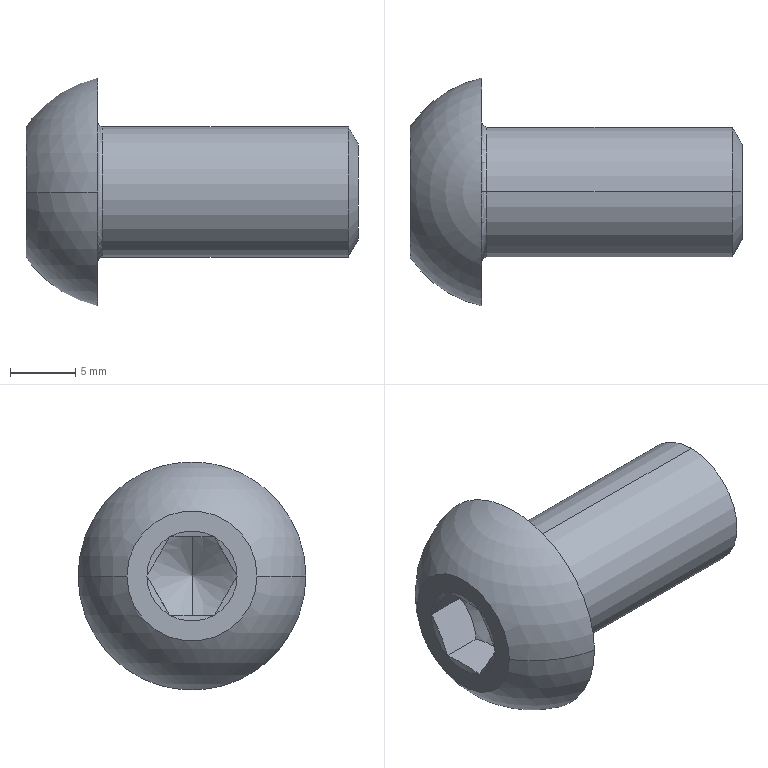Part | SolidWorks | 1 solid | 25 faces | box 25.5 x 17.5 x 17.5 mm | volume 2396 mm3 | cone 10 | plane 9 | torus 2 | sphere 2 | cylinder 2 | commonest cylinder face diameters 10 x2
STEP:
#1=CARTESIAN_POINT('',(0.,0.,3.701));
#2=VERTEX_POINT('',#1);
#3=CARTESIAN_POINT('',(0.,0.,-3.701));
#4=VERTEX_POINT('',#3);
#5=CARTESIAN_POINT('',(0.,0.,0.));
#6=DIRECTION('',(-1.,0.,0.));
#7=DIRECTION('',(0.,0.,1.));
#8=AXIS2_PLACEMENT_3D('',#5,#6,#7);
#9=CIRCLE('',#8,3.701);
#10=EDGE_CURVE('',#2,#4,#9,.T.);
#11=ORIENTED_EDGE('',*,*,#10,.T.);
#12=CARTESIAN_POINT('',(-0.75,0.,-5.));
#13=VERTEX_POINT('',#12);
#14=CARTESIAN_POINT('',(-0.75,0.,-5.));
#15=DIRECTION('',(-0.5,0.,-0.866));
#16=VECTOR('',#15,1000.);
#17=LINE('',#14,#16);
#18=EDGE_CURVE('',#4,#13,#17,.T.);
#19=ORIENTED_EDGE('',*,*,#18,.T.);
#20=CARTESIAN_POINT('',(-0.75,0.,5.));
#21=VERTEX_POINT('',#20);
#22=CARTESIAN_POINT('',(-0.75,0.,0.));
#23=DIRECTION('',(-1.,0.,0.));
#24=DIRECTION('',(0.,0.,1.));
#25=AXIS2_PLACEMENT_3D('',#22,#23,#24);
#26=CIRCLE('',#25,5.);
#27=EDGE_CURVE('',#21,#13,#26,.T.);
#28=ORIENTED_EDGE('',*,*,#27,.F.);
#29=CARTESIAN_POINT('',(-0.75,0.,5.));
#30=DIRECTION('',(-0.5,0.,0.866));
#31=VECTOR('',#30,1000.);
#32=LINE('',#29,#31);
#33=EDGE_CURVE('',#2,#21,#32,.T.);
#34=ORIENTED_EDGE('',*,*,#33,.F.);
#35=EDGE_LOOP('',(#11,#19,#28,#34));
#36=FACE_OUTER_BOUND('',#35,.T.);
#37=CARTESIAN_POINT('',(-0.75,0.,0.));
#38=DIRECTION('',(-1.,0.,0.));
#39=DIRECTION('',(0.,0.,1.));
#40=AXIS2_PLACEMENT_3D('',#37,#38,#39);
#41=CONICAL_SURFACE('',#40,5.,1.047);
#42=ADVANCED_FACE('',(#36),#41,.T.);
#43=CARTESIAN_POINT('',(-20.,0.,0.));
#44=VERTEX_POINT('',#43);
#45=CARTESIAN_POINT('',(-22.061,0.,3.));
#46=VERTEX_POINT('',#45);
#47=CARTESIAN_POINT('',(-22.38,0.,3.464));
#48=DIRECTION('',(-0.5663,0.,0.8242));
#49=VECTOR('',#48,1000.);
#50=LINE('',#47,#49);
#51=EDGE_CURVE('',#44,#46,#50,.T.);
#52=ORIENTED_EDGE('',*,*,#51,.F.);
#53=CARTESIAN_POINT('',(-22.061,0.,-3.));
#54=VERTEX_POINT('',#53);
#55=CARTESIAN_POINT('',(-22.38,0.,-3.464));
#56=DIRECTION('',(-0.5663,0.,-0.8242));
#57=VECTOR('',#56,1000.);
#58=LINE('',#55,#57);
#59=EDGE_CURVE('',#44,#54,#58,.T.);
#60=ORIENTED_EDGE('',*,*,#59,.T.);
#61=CARTESIAN_POINT('',(-22.38,-1.732,-3.));
#62=VERTEX_POINT('',#61);
#63=CARTESIAN_POINT('',(-22.061,0.,-3.));
#64=CARTESIAN_POINT('',(-22.061,-0.2941,-3.));
#65=CARTESIAN_POINT('',(-22.091,-0.5858,-3.));
#66=CARTESIAN_POINT('',(-22.203,-1.166,-3.));
#67=CARTESIAN_POINT('',(-22.284,-1.453,-3.));
#68=CARTESIAN_POINT('',(-22.38,-1.732,-3.));
#69=B_SPLINE_CURVE_WITH_KNOTS('',3,(#63,#64,#65,#66,#67,#68),.UNSPECIFIED.,.F.,.F.,(4,2,4),(0.01073,0.01162,0.0125),.UNSPECIFIED.);
#70=EDGE_CURVE('',#54,#62,#69,.T.);
#71=ORIENTED_EDGE('',*,*,#70,.T.);
#72=CARTESIAN_POINT('',(-22.38,-3.464,0.));
#73=VERTEX_POINT('',#72);
#74=CARTESIAN_POINT('',(-22.38,-1.732,-3.));
#75=CARTESIAN_POINT('',(-22.187,-2.012,-2.514));
#76=CARTESIAN_POINT('',(-22.062,-2.299,-2.019));
#77=CARTESIAN_POINT('',(-22.061,-2.669,-1.377));
#78=CARTESIAN_POINT('',(-22.068,-2.744,-1.247));
#79=CARTESIAN_POINT('',(-22.098,-2.891,-0.9922));
#80=CARTESIAN_POINT('',(-22.12,-2.964,-0.8658));
#81=CARTESIAN_POINT('',(-22.203,-3.181,-0.4899));
#82=CARTESIAN_POINT('',(-22.283,-3.324,-0.2435));
#83=CARTESIAN_POINT('',(-22.38,-3.464,0.));
#84=B_SPLINE_CURVE_WITH_KNOTS('',3,(#74,#75,#76,#77,#78,#79,#80,#81,#82,#83),.UNSPECIFIED.,.F.,.F.,(4,2,2,2,4),(0.000000241,0.001755,0.002194,0.002632,0.00351),.UNSPECIFIED.);
#85=EDGE_CURVE('',#62,#73,#84,.T.);
#86=ORIENTED_EDGE('',*,*,#85,.T.);
#87=CARTESIAN_POINT('',(-22.38,-1.732,3.));
#88=VERTEX_POINT('',#87);
#89=CARTESIAN_POINT('',(-22.38,-3.464,0.));
#90=CARTESIAN_POINT('',(-22.187,-3.184,0.4857));
#91=CARTESIAN_POINT('',(-22.062,-2.898,0.9812));
#92=CARTESIAN_POINT('',(-22.061,-2.527,1.623));
#93=CARTESIAN_POINT('',(-22.068,-2.452,1.753));
#94=CARTESIAN_POINT('',(-22.098,-2.305,2.008));
#95=CARTESIAN_POINT('',(-22.12,-2.232,2.134));
#96=CARTESIAN_POINT('',(-22.203,-2.015,2.51));
#97=CARTESIAN_POINT('',(-22.283,-1.873,2.756));
#98=CARTESIAN_POINT('',(-22.38,-1.732,3.));
#99=B_SPLINE_CURVE_WITH_KNOTS('',3,(#89,#90,#91,#92,#93,#94,#95,#96,#97,#98),.UNSPECIFIED.,.F.,.F.,(4,2,2,2,4),(0.000000241,0.001755,0.002194,0.002632,0.00351),.UNSPECIFIED.);
#100=EDGE_CURVE('',#73,#88,#99,.T.);
#101=ORIENTED_EDGE('',*,*,#100,.T.);
#102=CARTESIAN_POINT('',(-22.38,-1.732,3.));
#103=CARTESIAN_POINT('',(-22.284,-1.453,3.));
#104=CARTESIAN_POINT('',(-22.203,-1.166,3.));
#105=CARTESIAN_POINT('',(-22.091,-0.5858,3.));
#106=CARTESIAN_POINT('',(-22.061,-0.2941,3.));
#107=CARTESIAN_POINT('',(-22.061,0.,3.));
#108=B_SPLINE_CURVE_WITH_KNOTS('',3,(#102,#103,#104,#105,#106,#107),.UNSPECIFIED.,.F.,.F.,(4,2,4),(0.002487,0.003368,0.00425),.UNSPECIFIED.);
#109=EDGE_CURVE('',#88,#46,#108,.T.);
#110=ORIENTED_EDGE('',*,*,#109,.T.);
#111=EDGE_LOOP('',(#52,#60,#71,#86,#101,#110));
#112=FACE_OUTER_BOUND('',#111,.T.);
#113=CARTESIAN_POINT('',(-22.38,0.,0.));
#114=DIRECTION('',(-1.,0.,0.));
#115=DIRECTION('',(0.,0.,1.));
#116=AXIS2_PLACEMENT_3D('',#113,#114,#115);
#117=CONICAL_SURFACE('',#116,3.464,0.9688);
#118=ADVANCED_FACE('',(#112),#117,.F.);
#119=CARTESIAN_POINT('',(-20.,0.,-5.4));
#120=VERTEX_POINT('',#119);
#121=CARTESIAN_POINT('',(-20.,0.,5.4));
#122=VERTEX_POINT('',#121);
#123=CARTESIAN_POINT('',(-20.,0.,0.));
#124=DIRECTION('',(-1.,0.,0.));
#125=DIRECTION('',(0.,0.,1.));
#126=AXIS2_PLACEMENT_3D('',#123,#124,#125);
#127=CIRCLE('',#126,5.4);
#128=EDGE_CURVE('',#120,#122,#127,.T.);
#129=ORIENTED_EDGE('',*,*,#128,.F.);
#130=CARTESIAN_POINT('',(-19.6,0.,-5.));
#131=VERTEX_POINT('',#130);
#132=CARTESIAN_POINT('',(-19.6,0.,-5.4));
#133=DIRECTION('',(0.,1.,0.));
#134=DIRECTION('',(0.,0.,1.));
#135=AXIS2_PLACEMENT_3D('',#132,#133,#134);
#136=CIRCLE('',#135,0.4);
#137=EDGE_CURVE('',#120,#131,#136,.T.);
#138=ORIENTED_EDGE('',*,*,#137,.T.);
#139=CARTESIAN_POINT('',(-19.6,0.,5.));
#140=VERTEX_POINT('',#139);
#141=CARTESIAN_POINT('',(-19.6,0.,0.));
#142=DIRECTION('',(-1.,0.,0.));
#143=DIRECTION('',(0.,0.,1.));
#144=AXIS2_PLACEMENT_3D('',#141,#142,#143);
#145=CIRCLE('',#144,5.);
#146=EDGE_CURVE('',#131,#140,#145,.T.);
#147=ORIENTED_EDGE('',*,*,#146,.T.);
#148=CARTESIAN_POINT('',(-19.6,0.,5.4));
#149=DIRECTION('',(0.,-1.,0.));
#150=DIRECTION('',(0.,0.,-1.));
#151=AXIS2_PLACEMENT_3D('',#148,#149,#150);
#152=CIRCLE('',#151,0.4);
#153=EDGE_CURVE('',#122,#140,#152,.T.);
#154=ORIENTED_EDGE('',*,*,#153,.F.);
#155=EDGE_LOOP('',(#129,#138,#147,#154));
#156=FACE_OUTER_BOUND('',#155,.T.);
#157=CARTESIAN_POINT('',(-19.6,0.,0.));
#158=DIRECTION('',(-1.,0.,0.));
#159=DIRECTION('',(0.,0.,1.));
#160=AXIS2_PLACEMENT_3D('',#157,#158,#159);
#161=TOROIDAL_SURFACE('',#160,5.4,0.4);
#162=ADVANCED_FACE('',(#156),#161,.F.);
#163=CARTESIAN_POINT('',(-20.,8.75,0.));
#164=VERTEX_POINT('',#163);
#165=CARTESIAN_POINT('',(-20.,-8.75,0.));
#166=VERTEX_POINT('',#165);
#167=CARTESIAN_POINT('',(-20.,0.,0.));
#168=DIRECTION('',(-1.,0.,0.));
#169=DIRECTION('',(0.,0.,1.));
#170=AXIS2_PLACEMENT_3D('',#167,#168,#169);
#171=CIRCLE('',#170,8.75);
#172=EDGE_CURVE('',#164,#166,#171,.T.);
#173=ORIENTED_EDGE('',*,*,#172,.T.);
#174=CARTESIAN_POINT('',(-25.5,-5.,0.));
#175=VERTEX_POINT('',#174);
#176=CARTESIAN_POINT('',(-18.062,0.,0.));
#177=DIRECTION('',(0.,0.,-1.));
#178=DIRECTION('',(0.,1.,0.));
#179=AXIS2_PLACEMENT_3D('',#176,#177,#178);
#180=CIRCLE('',#179,8.962);
#181=EDGE_CURVE('',#166,#175,#180,.T.);
#182=ORIENTED_EDGE('',*,*,#181,.T.);
#183=CARTESIAN_POINT('',(-25.5,5.,0.));
#184=VERTEX_POINT('',#183);
#185=CARTESIAN_POINT('',(-25.5,0.,0.));
#186=DIRECTION('',(-1.,0.,0.));
#187=DIRECTION('',(0.,0.,1.));
#188=AXIS2_PLACEMENT_3D('',#185,#186,#187);
#189=CIRCLE('',#188,5.);
#190=EDGE_CURVE('',#184,#175,#189,.T.);
#191=ORIENTED_EDGE('',*,*,#190,.F.);
#192=CARTESIAN_POINT('',(-18.062,0.,0.));
#193=DIRECTION('',(0.,0.,1.));
#194=DIRECTION('',(1.,0.,0.));
#195=AXIS2_PLACEMENT_3D('',#192,#193,#194);
#196=CIRCLE('',#195,8.962);
#197=EDGE_CURVE('',#164,#184,#196,.T.);
#198=ORIENTED_EDGE('',*,*,#197,.F.);
#199=EDGE_LOOP('',(#173,#182,#191,#198));
#200=FACE_OUTER_BOUND('',#199,.T.);
#201=CARTESIAN_POINT('',(-18.062,0.,0.));
#202=DIRECTION('',(0.,0.,-1.));
#203=DIRECTION('',(0.,1.,0.));
#204=AXIS2_PLACEMENT_3D('',#201,#202,#203);
#205=SPHERICAL_SURFACE('',#204,8.962);
#206=ADVANCED_FACE('',(#200),#205,.T.);
#207=ORIENTED_EDGE('',*,*,#27,.T.);
#208=CARTESIAN_POINT('',(-25.5,0.,-5.));
#209=DIRECTION('',(-1.,0.,0.));
#210=VECTOR('',#209,1000.);
#211=LINE('',#208,#210);
#212=EDGE_CURVE('',#13,#131,#211,.T.);
#213=ORIENTED_EDGE('',*,*,#212,.T.);
#214=CARTESIAN_POINT('',(-19.6,0.,0.));
#215=DIRECTION('',(-1.,0.,0.));
#216=DIRECTION('',(0.,0.,1.));
#217=AXIS2_PLACEMENT_3D('',#214,#215,#216);
#218=CIRCLE('',#217,5.);
#219=EDGE_CURVE('',#140,#131,#218,.T.);
#220=ORIENTED_EDGE('',*,*,#219,.F.);
#221=CARTESIAN_POINT('',(-25.5,0.,5.));
#222=DIRECTION('',(-1.,0.,0.));
#223=VECTOR('',#222,1000.);
#224=LINE('',#221,#223);
#225=EDGE_CURVE('',#21,#140,#224,.T.);
#226=ORIENTED_EDGE('',*,*,#225,.F.);
#227=EDGE_LOOP('',(#207,#213,#220,#226));
#228=FACE_OUTER_BOUND('',#227,.T.);
#229=CARTESIAN_POINT('',(-25.5,0.,0.));
#230=DIRECTION('',(-1.,0.,0.));
#231=DIRECTION('',(0.,0.,1.));
#232=AXIS2_PLACEMENT_3D('',#229,#230,#231);
#233=CYLINDRICAL_SURFACE('',#232,5.);
#234=ADVANCED_FACE('',(#228),#233,.T.);
#235=ORIENTED_EDGE('',*,*,#212,.F.);
#236=CARTESIAN_POINT('',(-0.75,0.,0.));
#237=DIRECTION('',(-1.,0.,0.));
#238=DIRECTION('',(0.,0.,1.));
#239=AXIS2_PLACEMENT_3D('',#236,#237,#238);
#240=CIRCLE('',#239,5.);
#241=EDGE_CURVE('',#13,#21,#240,.T.);
#242=ORIENTED_EDGE('',*,*,#241,.T.);
#243=ORIENTED_EDGE('',*,*,#225,.T.);
#244=ORIENTED_EDGE('',*,*,#146,.F.);
#245=EDGE_LOOP('',(#235,#242,#243,#244));
#246=FACE_OUTER_BOUND('',#245,.T.);
#247=CARTESIAN_POINT('',(-25.5,0.,0.));
#248=DIRECTION('',(-1.,0.,0.));
#249=DIRECTION('',(0.,0.,1.));
#250=AXIS2_PLACEMENT_3D('',#247,#248,#249);
#251=CYLINDRICAL_SURFACE('',#250,5.);
#252=ADVANCED_FACE('',(#246),#251,.T.);
#253=ORIENTED_EDGE('',*,*,#190,.T.);
#254=CARTESIAN_POINT('',(-25.5,0.,0.));
#255=DIRECTION('',(-1.,0.,0.));
#256=DIRECTION('',(0.,0.,1.));
#257=AXIS2_PLACEMENT_3D('',#254,#255,#256);
#258=CIRCLE('',#257,5.);
#259=EDGE_CURVE('',#175,#184,#258,.T.);
#260=ORIENTED_EDGE('',*,*,#259,.T.);
#261=EDGE_LOOP('',(#253,#260));
#262=FACE_OUTER_BOUND('',#261,.T.);
#263=CARTESIAN_POINT('',(-25.5,-1.732,-3.));
#264=VERTEX_POINT('',#263);
#265=CARTESIAN_POINT('',(-25.5,-3.464,0.));
#266=VERTEX_POINT('',#265);
#267=CARTESIAN_POINT('',(-25.5,0.,0.));
#268=DIRECTION('',(-1.,0.,0.));
#269=DIRECTION('',(0.,0.,-1.));
#270=AXIS2_PLACEMENT_3D('',#267,#268,#269);
#271=CIRCLE('',#270,3.464);
#272=EDGE_CURVE('',#264,#266,#271,.T.);
#273=ORIENTED_EDGE('',*,*,#272,.F.);
#274=CARTESIAN_POINT('',(-25.5,1.732,-3.));
#275=VERTEX_POINT('',#274);
#276=CARTESIAN_POINT('',(-25.5,0.,0.));
#277=DIRECTION('',(-1.,0.,0.));
#278=DIRECTION('',(0.,0.,-1.));
#279=AXIS2_PLACEMENT_3D('',#276,#277,#278);
#280=CIRCLE('',#279,3.464);
#281=EDGE_CURVE('',#275,#264,#280,.T.);
#282=ORIENTED_EDGE('',*,*,#281,.F.);
#283=CARTESIAN_POINT('',(-25.5,3.464,0.));
#284=VERTEX_POINT('',#283);
#285=CARTESIAN_POINT('',(-25.5,0.,0.));
#286=DIRECTION('',(-1.,0.,0.));
#287=DIRECTION('',(0.,0.,-1.));
#288=AXIS2_PLACEMENT_3D('',#285,#286,#287);
#289=CIRCLE('',#288,3.464);
#290=EDGE_CURVE('',#284,#275,#289,.T.);
#291=ORIENTED_EDGE('',*,*,#290,.F.);
#292=CARTESIAN_POINT('',(-25.5,1.732,3.));
#293=VERTEX_POINT('',#292);
#294=CARTESIAN_POINT('',(-25.5,0.,0.));
#295=DIRECTION('',(-1.,0.,0.));
#296=DIRECTION('',(0.,0.,-1.));
#297=AXIS2_PLACEMENT_3D('',#294,#295,#296);
#298=CIRCLE('',#297,3.464);
#299=EDGE_CURVE('',#293,#284,#298,.T.);
#300=ORIENTED_EDGE('',*,*,#299,.F.);
#301=CARTESIAN_POINT('',(-25.5,-1.732,3.));
#302=VERTEX_POINT('',#301);
#303=CARTESIAN_POINT('',(-25.5,0.,0.));
#304=DIRECTION('',(-1.,0.,0.));
#305=DIRECTION('',(0.,0.,-1.));
#306=AXIS2_PLACEMENT_3D('',#303,#304,#305);
#307=CIRCLE('',#306,3.464);
#308=EDGE_CURVE('',#302,#293,#307,.T.);
#309=ORIENTED_EDGE('',*,*,#308,.F.);
#310=CARTESIAN_POINT('',(-25.5,0.,0.));
#311=DIRECTION('',(-1.,0.,0.));
#312=DIRECTION('',(0.,-1.,0.));
#313=AXIS2_PLACEMENT_3D('',#310,#311,#312);
#314=CIRCLE('',#313,3.464);
#315=EDGE_CURVE('',#266,#302,#314,.T.);
#316=ORIENTED_EDGE('',*,*,#315,.F.);
#317=EDGE_LOOP('',(#273,#282,#291,#300,#309,#316));
#318=FACE_BOUND('',#317,.T.);
#319=CARTESIAN_POINT('',(-25.5,0.,0.));
#320=DIRECTION('',(1.,0.,0.));
#321=DIRECTION('',(0.,0.,-1.));
#322=AXIS2_PLACEMENT_3D('',#319,#320,#321);
#323=PLANE('',#322);
#324=ADVANCED_FACE('',(#262,#318),#323,.F.);
#325=ORIENTED_EDGE('',*,*,#181,.F.);
#326=CARTESIAN_POINT('',(-20.,0.,0.));
#327=DIRECTION('',(-1.,0.,0.));
#328=DIRECTION('',(0.,0.,1.));
#329=AXIS2_PLACEMENT_3D('',#326,#327,#328);
#330=CIRCLE('',#329,8.75);
#331=EDGE_CURVE('',#166,#164,#330,.T.);
#332=ORIENTED_EDGE('',*,*,#331,.T.);
#333=ORIENTED_EDGE('',*,*,#197,.T.);
#334=ORIENTED_EDGE('',*,*,#259,.F.);
#335=EDGE_LOOP('',(#325,#332,#333,#334));
#336=FACE_OUTER_BOUND('',#335,.T.);
#337=CARTESIAN_POINT('',(-18.062,0.,0.));
#338=DIRECTION('',(0.,0.,-1.));
#339=DIRECTION('',(0.,1.,0.));
#340=AXIS2_PLACEMENT_3D('',#337,#338,#339);
#341=SPHERICAL_SURFACE('',#340,8.962);
#342=ADVANCED_FACE('',(#336),#341,.T.);
#343=ORIENTED_EDGE('',*,*,#172,.F.);
#344=ORIENTED_EDGE('',*,*,#331,.F.);
#345=EDGE_LOOP('',(#343,#344));
#346=FACE_OUTER_BOUND('',#345,.T.);
#347=CARTESIAN_POINT('',(-20.,0.,0.));
#348=DIRECTION('',(-1.,0.,0.));
#349=DIRECTION('',(0.,0.,1.));
#350=AXIS2_PLACEMENT_3D('',#347,#348,#349);
#351=CIRCLE('',#350,5.4);
#352=EDGE_CURVE('',#122,#120,#351,.T.);
#353=ORIENTED_EDGE('',*,*,#352,.T.);
#354=ORIENTED_EDGE('',*,*,#128,.T.);
#355=EDGE_LOOP('',(#353,#354));
#356=FACE_BOUND('',#355,.T.);
#357=CARTESIAN_POINT('',(-20.,5.4,0.));
#358=DIRECTION('',(-1.,0.,0.));
#359=DIRECTION('',(0.,0.,1.));
#360=AXIS2_PLACEMENT_3D('',#357,#358,#359);
#361=PLANE('',#360);
#362=ADVANCED_FACE('',(#346,#356),#361,.F.);
#363=ORIENTED_EDGE('',*,*,#137,.F.);
#364=ORIENTED_EDGE('',*,*,#352,.F.);
#365=ORIENTED_EDGE('',*,*,#153,.T.);
#366=ORIENTED_EDGE('',*,*,#219,.T.);
#367=EDGE_LOOP('',(#363,#364,#365,#366));
#368=FACE_OUTER_BOUND('',#367,.T.);
#369=CARTESIAN_POINT('',(-19.6,0.,0.));
#370=DIRECTION('',(-1.,0.,0.));
#371=DIRECTION('',(0.,0.,1.));
#372=AXIS2_PLACEMENT_3D('',#369,#370,#371);
#373=TOROIDAL_SURFACE('',#372,5.4,0.4);
#374=ADVANCED_FACE('',(#368),#373,.F.);
#375=CARTESIAN_POINT('',(-25.5,-1.732,-3.));
#376=CARTESIAN_POINT('',(-25.428,-1.155,-3.));
#377=CARTESIAN_POINT('',(-25.385,-0.5749,-3.));
#378=CARTESIAN_POINT('',(-25.385,0.5803,-3.));
#379=CARTESIAN_POINT('',(-25.429,1.157,-3.));
#380=CARTESIAN_POINT('',(-25.5,1.732,-3.));
#381=B_SPLINE_CURVE_WITH_KNOTS('',3,(#375,#376,#377,#378,#379,#380),.UNSPECIFIED.,.F.,.F.,(4,2,4),(0.002838,0.00458,0.006321),.UNSPECIFIED.);
#382=EDGE_CURVE('',#264,#275,#381,.T.);
#383=ORIENTED_EDGE('',*,*,#382,.T.);
#384=ORIENTED_EDGE('',*,*,#281,.T.);
#385=EDGE_LOOP('',(#383,#384));
#386=FACE_OUTER_BOUND('',#385,.T.);
#387=CARTESIAN_POINT('',(-1024.64,0.,0.));
#388=DIRECTION('',(-1.,0.,0.));
#389=DIRECTION('',(0.,-1.,0.));
#390=AXIS2_PLACEMENT_3D('',#387,#388,#389);
#391=CONICAL_SURFACE('',#390,4028.025,1.327);
#392=ADVANCED_FACE('',(#386),#391,.F.);
#393=CARTESIAN_POINT('',(-25.5,1.732,-3.));
#394=CARTESIAN_POINT('',(-25.428,2.021,-2.5));
#395=CARTESIAN_POINT('',(-25.341,2.598,-1.5));
#396=CARTESIAN_POINT('',(-25.428,3.175,-0.5));
#397=CARTESIAN_POINT('',(-25.5,3.464,0.));
#398=B_SPLINE_CURVE_WITH_KNOTS('',3,(#393,#394,#395,#396,#397),.UNSPECIFIED.,.F.,.F.,(4,1,4),(0.000000231,0.001732,0.003464),.UNSPECIFIED.);
#399=EDGE_CURVE('',#275,#284,#398,.T.);
#400=ORIENTED_EDGE('',*,*,#399,.T.);
#401=ORIENTED_EDGE('',*,*,#290,.T.);
#402=EDGE_LOOP('',(#400,#401));
#403=FACE_OUTER_BOUND('',#402,.T.);
#404=CARTESIAN_POINT('',(-1024.64,0.,0.));
#405=DIRECTION('',(-1.,0.,0.));
#406=DIRECTION('',(0.,-1.,0.));
#407=AXIS2_PLACEMENT_3D('',#404,#405,#406);
#408=CONICAL_SURFACE('',#407,4028.025,1.327);
#409=ADVANCED_FACE('',(#403),#408,.F.);
#410=CARTESIAN_POINT('',(-25.5,3.464,0.));
#411=CARTESIAN_POINT('',(-25.428,3.175,0.5));
#412=CARTESIAN_POINT('',(-25.341,2.598,1.5));
#413=CARTESIAN_POINT('',(-25.428,2.021,2.5));
#414=CARTESIAN_POINT('',(-25.5,1.732,3.));
#415=B_SPLINE_CURVE_WITH_KNOTS('',3,(#410,#411,#412,#413,#414),.UNSPECIFIED.,.F.,.F.,(4,1,4),(0.000000231,0.001732,0.003464),.UNSPECIFIED.);
#416=EDGE_CURVE('',#284,#293,#415,.T.);
#417=ORIENTED_EDGE('',*,*,#416,.T.);
#418=ORIENTED_EDGE('',*,*,#299,.T.);
#419=EDGE_LOOP('',(#417,#418));
#420=FACE_OUTER_BOUND('',#419,.T.);
#421=CARTESIAN_POINT('',(-1024.64,0.,0.));
#422=DIRECTION('',(-1.,0.,0.));
#423=DIRECTION('',(0.,-1.,0.));
#424=AXIS2_PLACEMENT_3D('',#421,#422,#423);
#425=CONICAL_SURFACE('',#424,4028.025,1.327);
#426=ADVANCED_FACE('',(#420),#425,.F.);
#427=CARTESIAN_POINT('',(-25.5,1.732,3.));
#428=CARTESIAN_POINT('',(-25.429,1.157,3.));
#429=CARTESIAN_POINT('',(-25.385,0.5803,3.));
#430=CARTESIAN_POINT('',(-25.385,-0.5749,3.));
#431=CARTESIAN_POINT('',(-25.428,-1.155,3.));
#432=CARTESIAN_POINT('',(-25.5,-1.732,3.));
#433=B_SPLINE_CURVE_WITH_KNOTS('',3,(#427,#428,#429,#430,#431,#432),.UNSPECIFIED.,.F.,.F.,(4,2,4),(0.007099,0.008838,0.01058),.UNSPECIFIED.);
#434=EDGE_CURVE('',#293,#302,#433,.T.);
#435=ORIENTED_EDGE('',*,*,#434,.T.);
#436=ORIENTED_EDGE('',*,*,#308,.T.);
#437=EDGE_LOOP('',(#435,#436));
#438=FACE_OUTER_BOUND('',#437,.T.);
#439=CARTESIAN_POINT('',(-1024.64,0.,0.));
#440=DIRECTION('',(-1.,0.,0.));
#441=DIRECTION('',(0.,-1.,0.));
#442=AXIS2_PLACEMENT_3D('',#439,#440,#441);
#443=CONICAL_SURFACE('',#442,4028.025,1.327);
#444=ADVANCED_FACE('',(#438),#443,.F.);
#445=CARTESIAN_POINT('',(-25.5,-1.732,3.));
#446=CARTESIAN_POINT('',(-25.428,-2.021,2.5));
#447=CARTESIAN_POINT('',(-25.341,-2.598,1.5));
#448=CARTESIAN_POINT('',(-25.428,-3.175,0.5));
#449=CARTESIAN_POINT('',(-25.5,-3.464,0.));
#450=B_SPLINE_CURVE_WITH_KNOTS('',3,(#445,#446,#447,#448,#449),.UNSPECIFIED.,.F.,.F.,(4,1,4),(0.000000231,0.001732,0.003464),.UNSPECIFIED.);
#451=EDGE_CURVE('',#302,#266,#450,.T.);
#452=ORIENTED_EDGE('',*,*,#451,.T.);
#453=ORIENTED_EDGE('',*,*,#315,.T.);
#454=EDGE_LOOP('',(#452,#453));
#455=FACE_OUTER_BOUND('',#454,.T.);
#456=CARTESIAN_POINT('',(-1024.64,0.,0.));
#457=DIRECTION('',(-1.,0.,0.));
#458=DIRECTION('',(0.,-1.,0.));
#459=AXIS2_PLACEMENT_3D('',#456,#457,#458);
#460=CONICAL_SURFACE('',#459,4028.025,1.327);
#461=ADVANCED_FACE('',(#455),#460,.F.);
#462=CARTESIAN_POINT('',(-25.5,-3.464,0.));
#463=CARTESIAN_POINT('',(-25.428,-3.175,-0.5));
#464=CARTESIAN_POINT('',(-25.341,-2.598,-1.5));
#465=CARTESIAN_POINT('',(-25.428,-2.021,-2.5));
#466=CARTESIAN_POINT('',(-25.5,-1.732,-3.));
#467=B_SPLINE_CURVE_WITH_KNOTS('',3,(#462,#463,#464,#465,#466),.UNSPECIFIED.,.F.,.F.,(4,1,4),(0.000000231,0.001732,0.003464),.UNSPECIFIED.);
#468=EDGE_CURVE('',#266,#264,#467,.T.);
#469=ORIENTED_EDGE('',*,*,#468,.T.);
#470=ORIENTED_EDGE('',*,*,#272,.T.);
#471=EDGE_LOOP('',(#469,#470));
#472=FACE_OUTER_BOUND('',#471,.T.);
#473=CARTESIAN_POINT('',(-1024.64,0.,0.));
#474=DIRECTION('',(-1.,0.,0.));
#475=DIRECTION('',(0.,-1.,0.));
#476=AXIS2_PLACEMENT_3D('',#473,#474,#475);
#477=CONICAL_SURFACE('',#476,4028.025,1.327);
#478=ADVANCED_FACE('',(#472),#477,.F.);
#479=ORIENTED_EDGE('',*,*,#59,.F.);
#480=ORIENTED_EDGE('',*,*,#51,.T.);
#481=CARTESIAN_POINT('',(-22.38,1.732,3.));
#482=VERTEX_POINT('',#481);
#483=CARTESIAN_POINT('',(-22.061,0.,3.));
#484=CARTESIAN_POINT('',(-22.061,0.2938,3.));
#485=CARTESIAN_POINT('',(-22.092,0.5926,3.));
#486=CARTESIAN_POINT('',(-22.205,1.172,3.));
#487=CARTESIAN_POINT('',(-22.285,1.454,3.));
#488=CARTESIAN_POINT('',(-22.38,1.732,3.));
#489=B_SPLINE_CURVE_WITH_KNOTS('',3,(#483,#484,#485,#486,#487,#488),.UNSPECIFIED.,.F.,.F.,(4,2,4),(0.00425,0.00513,0.00601),.UNSPECIFIED.);
#490=EDGE_CURVE('',#46,#482,#489,.T.);
#491=ORIENTED_EDGE('',*,*,#490,.T.);
#492=CARTESIAN_POINT('',(-22.38,3.464,0.));
#493=VERTEX_POINT('',#492);
#494=CARTESIAN_POINT('',(-22.38,1.732,3.));
#495=CARTESIAN_POINT('',(-22.187,2.012,2.514));
#496=CARTESIAN_POINT('',(-22.062,2.299,2.019));
#497=CARTESIAN_POINT('',(-22.061,2.669,1.377));
#498=CARTESIAN_POINT('',(-22.068,2.744,1.247));
#499=CARTESIAN_POINT('',(-22.098,2.891,0.9922));
#500=CARTESIAN_POINT('',(-22.12,2.964,0.8658));
#501=CARTESIAN_POINT('',(-22.203,3.181,0.4899));
#502=CARTESIAN_POINT('',(-22.283,3.324,0.2435));
#503=CARTESIAN_POINT('',(-22.38,3.464,0.));
#504=B_SPLINE_CURVE_WITH_KNOTS('',3,(#494,#495,#496,#497,#498,#499,#500,#501,#502,#503),.UNSPECIFIED.,.F.,.F.,(4,2,2,2,4),(0.000000241,0.001755,0.002194,0.002632,0.00351),.UNSPECIFIED.);
#505=EDGE_CURVE('',#482,#493,#504,.T.);
#506=ORIENTED_EDGE('',*,*,#505,.T.);
#507=CARTESIAN_POINT('',(-22.38,1.732,-3.));
#508=VERTEX_POINT('',#507);
#509=CARTESIAN_POINT('',(-22.38,3.464,0.));
#510=CARTESIAN_POINT('',(-22.187,3.184,-0.4857));
#511=CARTESIAN_POINT('',(-22.062,2.898,-0.9812));
#512=CARTESIAN_POINT('',(-22.061,2.527,-1.623));
#513=CARTESIAN_POINT('',(-22.068,2.452,-1.753));
#514=CARTESIAN_POINT('',(-22.098,2.305,-2.008));
#515=CARTESIAN_POINT('',(-22.12,2.232,-2.134));
#516=CARTESIAN_POINT('',(-22.203,2.015,-2.51));
#517=CARTESIAN_POINT('',(-22.283,1.873,-2.756));
#518=CARTESIAN_POINT('',(-22.38,1.732,-3.));
#519=B_SPLINE_CURVE_WITH_KNOTS('',3,(#509,#510,#511,#512,#513,#514,#515,#516,#517,#518),.UNSPECIFIED.,.F.,.F.,(4,2,2,2,4),(0.000000241,0.001755,0.002194,0.002632,0.00351),.UNSPECIFIED.);
#520=EDGE_CURVE('',#493,#508,#519,.T.);
#521=ORIENTED_EDGE('',*,*,#520,.T.);
#522=CARTESIAN_POINT('',(-22.38,1.732,-3.));
#523=CARTESIAN_POINT('',(-22.285,1.454,-3.));
#524=CARTESIAN_POINT('',(-22.205,1.172,-3.));
#525=CARTESIAN_POINT('',(-22.092,0.5926,-3.));
#526=CARTESIAN_POINT('',(-22.061,0.2938,-3.));
#527=CARTESIAN_POINT('',(-22.061,0.,-3.));
#528=B_SPLINE_CURVE_WITH_KNOTS('',3,(#522,#523,#524,#525,#526,#527),.UNSPECIFIED.,.F.,.F.,(4,2,4),(0.008971,0.009852,0.01073),.UNSPECIFIED.);
#529=EDGE_CURVE('',#508,#54,#528,.T.);
#530=ORIENTED_EDGE('',*,*,#529,.T.);
#531=EDGE_LOOP('',(#479,#480,#491,#506,#521,#530));
#532=FACE_OUTER_BOUND('',#531,.T.);
#533=CARTESIAN_POINT('',(-22.38,0.,0.));
#534=DIRECTION('',(-1.,0.,0.));
#535=DIRECTION('',(0.,0.,1.));
#536=AXIS2_PLACEMENT_3D('',#533,#534,#535);
#537=CONICAL_SURFACE('',#536,3.464,0.9688);
#538=ADVANCED_FACE('',(#532),#537,.F.);
#539=ORIENTED_EDGE('',*,*,#399,.F.);
#540=CARTESIAN_POINT('',(-20.,1.732,-3.));
#541=DIRECTION('',(-1.,0.,0.));
#542=VECTOR('',#541,1000.);
#543=LINE('',#540,#542);
#544=EDGE_CURVE('',#508,#275,#543,.T.);
#545=ORIENTED_EDGE('',*,*,#544,.F.);
#546=ORIENTED_EDGE('',*,*,#520,.F.);
#547=CARTESIAN_POINT('',(-20.,3.464,0.));
#548=DIRECTION('',(-1.,0.,0.));
#549=VECTOR('',#548,1000.);
#550=LINE('',#547,#549);
#551=EDGE_CURVE('',#493,#284,#550,.T.);
#552=ORIENTED_EDGE('',*,*,#551,.T.);
#553=EDGE_LOOP('',(#539,#545,#546,#552));
#554=FACE_OUTER_BOUND('',#553,.T.);
#555=CARTESIAN_POINT('',(-20.,3.464,0.));
#556=DIRECTION('',(0.,0.866,-0.5));
#557=DIRECTION('',(0.,0.5,0.866));
#558=AXIS2_PLACEMENT_3D('',#555,#556,#557);
#559=PLANE('',#558);
#560=ADVANCED_FACE('',(#554),#559,.F.);
#561=ORIENTED_EDGE('',*,*,#382,.F.);
#562=CARTESIAN_POINT('',(-20.,-1.732,-3.));
#563=DIRECTION('',(-1.,0.,0.));
#564=VECTOR('',#563,1000.);
#565=LINE('',#562,#564);
#566=EDGE_CURVE('',#62,#264,#565,.T.);
#567=ORIENTED_EDGE('',*,*,#566,.F.);
#568=ORIENTED_EDGE('',*,*,#70,.F.);
#569=ORIENTED_EDGE('',*,*,#529,.F.);
#570=ORIENTED_EDGE('',*,*,#544,.T.);
#571=EDGE_LOOP('',(#561,#567,#568,#569,#570));
#572=FACE_OUTER_BOUND('',#571,.T.);
#573=CARTESIAN_POINT('',(-20.,1.732,-3.));
#574=DIRECTION('',(0.,0.,-1.));
#575=DIRECTION('',(-1.,0.,0.));
#576=AXIS2_PLACEMENT_3D('',#573,#574,#575);
#577=PLANE('',#576);
#578=ADVANCED_FACE('',(#572),#577,.F.);
#579=ORIENTED_EDGE('',*,*,#468,.F.);
#580=CARTESIAN_POINT('',(-20.,-3.464,0.));
#581=DIRECTION('',(-1.,0.,0.));
#582=VECTOR('',#581,1000.);
#583=LINE('',#580,#582);
#584=EDGE_CURVE('',#73,#266,#583,.T.);
#585=ORIENTED_EDGE('',*,*,#584,.F.);
#586=ORIENTED_EDGE('',*,*,#85,.F.);
#587=ORIENTED_EDGE('',*,*,#566,.T.);
#588=EDGE_LOOP('',(#579,#585,#586,#587));
#589=FACE_OUTER_BOUND('',#588,.T.);
#590=CARTESIAN_POINT('',(-20.,-1.732,-3.));
#591=DIRECTION('',(0.,-0.866,-0.5));
#592=DIRECTION('',(0.,0.5,-0.866));
#593=AXIS2_PLACEMENT_3D('',#590,#591,#592);
#594=PLANE('',#593);
#595=ADVANCED_FACE('',(#589),#594,.F.);
#596=ORIENTED_EDGE('',*,*,#451,.F.);
#597=CARTESIAN_POINT('',(-20.,-1.732,3.));
#598=DIRECTION('',(-1.,0.,0.));
#599=VECTOR('',#598,1000.);
#600=LINE('',#597,#599);
#601=EDGE_CURVE('',#88,#302,#600,.T.);
#602=ORIENTED_EDGE('',*,*,#601,.F.);
#603=ORIENTED_EDGE('',*,*,#100,.F.);
#604=ORIENTED_EDGE('',*,*,#584,.T.);
#605=EDGE_LOOP('',(#596,#602,#603,#604));
#606=FACE_OUTER_BOUND('',#605,.T.);
#607=CARTESIAN_POINT('',(-20.,-3.464,0.));
#608=DIRECTION('',(0.,-0.866,0.5));
#609=DIRECTION('',(0.,-0.5,-0.866));
#610=AXIS2_PLACEMENT_3D('',#607,#608,#609);
#611=PLANE('',#610);
#612=ADVANCED_FACE('',(#606),#611,.F.);
#613=ORIENTED_EDGE('',*,*,#434,.F.);
#614=CARTESIAN_POINT('',(-20.,1.732,3.));
#615=DIRECTION('',(-1.,0.,0.));
#616=VECTOR('',#615,1000.);
#617=LINE('',#614,#616);
#618=EDGE_CURVE('',#482,#293,#617,.T.);
#619=ORIENTED_EDGE('',*,*,#618,.F.);
#620=ORIENTED_EDGE('',*,*,#490,.F.);
#621=ORIENTED_EDGE('',*,*,#109,.F.);
#622=ORIENTED_EDGE('',*,*,#601,.T.);
#623=EDGE_LOOP('',(#613,#619,#620,#621,#622));
#624=FACE_OUTER_BOUND('',#623,.T.);
#625=CARTESIAN_POINT('',(-20.,-1.732,3.));
#626=DIRECTION('',(0.,0.,1.));
#627=DIRECTION('',(0.,-1.,0.));
#628=AXIS2_PLACEMENT_3D('',#625,#626,#627);
#629=PLANE('',#628);
#630=ADVANCED_FACE('',(#624),#629,.F.);
#631=ORIENTED_EDGE('',*,*,#416,.F.);
#632=ORIENTED_EDGE('',*,*,#551,.F.);
#633=ORIENTED_EDGE('',*,*,#505,.F.);
#634=ORIENTED_EDGE('',*,*,#618,.T.);
#635=EDGE_LOOP('',(#631,#632,#633,#634));
#636=FACE_OUTER_BOUND('',#635,.T.);
#637=CARTESIAN_POINT('',(-20.,1.732,3.));
#638=DIRECTION('',(0.,0.866,0.5));
#639=DIRECTION('',(0.,-0.5,0.866));
#640=AXIS2_PLACEMENT_3D('',#637,#638,#639);
#641=PLANE('',#640);
#642=ADVANCED_FACE('',(#636),#641,.F.);
#643=ORIENTED_EDGE('',*,*,#18,.F.);
#644=CARTESIAN_POINT('',(0.,0.,0.));
#645=DIRECTION('',(-1.,0.,0.));
#646=DIRECTION('',(0.,0.,1.));
#647=AXIS2_PLACEMENT_3D('',#644,#645,#646);
#648=CIRCLE('',#647,3.701);
#649=EDGE_CURVE('',#4,#2,#648,.T.);
#650=ORIENTED_EDGE('',*,*,#649,.T.);
#651=ORIENTED_EDGE('',*,*,#33,.T.);
#652=ORIENTED_EDGE('',*,*,#241,.F.);
#653=EDGE_LOOP('',(#643,#650,#651,#652));
#654=FACE_OUTER_BOUND('',#653,.T.);
#655=CARTESIAN_POINT('',(-0.75,0.,0.));
#656=DIRECTION('',(-1.,0.,0.));
#657=DIRECTION('',(0.,0.,1.));
#658=AXIS2_PLACEMENT_3D('',#655,#656,#657);
#659=CONICAL_SURFACE('',#658,5.,1.047);
#660=ADVANCED_FACE('',(#654),#659,.T.);
#661=ORIENTED_EDGE('',*,*,#10,.F.);
#662=ORIENTED_EDGE('',*,*,#649,.F.);
#663=EDGE_LOOP('',(#661,#662));
#664=FACE_OUTER_BOUND('',#663,.T.);
#665=CARTESIAN_POINT('',(0.,5.,0.));
#666=DIRECTION('',(-1.,0.,0.));
#667=DIRECTION('',(0.,0.,1.));
#668=AXIS2_PLACEMENT_3D('',#665,#666,#667);
#669=PLANE('',#668);
#670=ADVANCED_FACE('',(#664),#669,.F.);
#671=CLOSED_SHELL('',(#42,#118,#162,#206,#234,#252,#324,#342,#362,#374,#392,#409,#426,#444,#461,#478,#538,#560,#578,#595,#612,#630,#642,#660,#670));
#672=MANIFOLD_SOLID_BREP('',#671);
#673=CARTESIAN_POINT('',(0.,0.,0.));
#674=DIRECTION('',(0.,0.,1.));
#675=DIRECTION('',(1.,0.,0.));
#676=AXIS2_PLACEMENT_3D('',#673,#674,#675);
#677=(LENGTH_UNIT()NAMED_UNIT(*)SI_UNIT(.MILLI.,.METRE.));
#678=UNCERTAINTY_MEASURE_WITH_UNIT(LENGTH_MEASURE(0.00001),#677,'','');
#679=(NAMED_UNIT(*)PLANE_ANGLE_UNIT()SI_UNIT($,.RADIAN.));
#680=(NAMED_UNIT(*)SI_UNIT($,.STERADIAN.)SOLID_ANGLE_UNIT());
#681=(GEOMETRIC_REPRESENTATION_CONTEXT(3)GLOBAL_UNCERTAINTY_ASSIGNED_CONTEXT((#678))GLOBAL_UNIT_ASSIGNED_CONTEXT((#677,#679,#680))REPRESENTATION_CONTEXT('',''));
#682=ADVANCED_BREP_SHAPE_REPRESENTATION('',(#672,#676),#681);